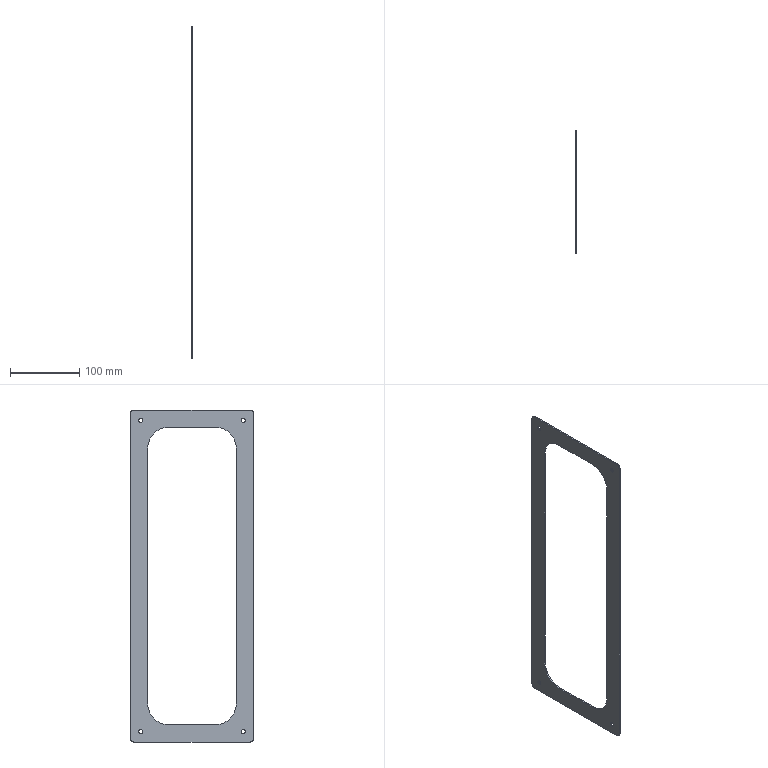Part | SolidWorks | features Fillet 2, ICE 2, Extrusion 1 | 1 solid | 26 faces | box 2 x 178 x 480 mm | volume 62076 mm3 | cylinder 16 | plane 10 | commonest cylinder face diameters 6 x8 10 x4 60 x4
STEP:
#1=CARTESIAN_POINT('',(0.,-74.,-222.));
#2=VERTEX_POINT('',#1);
#3=CARTESIAN_POINT('',(0.,-74.,-228.));
#4=VERTEX_POINT('',#3);
#5=CARTESIAN_POINT('',(0.,-74.,-225.));
#6=DIRECTION('',(1.,0.,0.));
#7=DIRECTION('',(0.,0.,-1.));
#8=AXIS2_PLACEMENT_3D('',#5,#6,#7);
#9=CIRCLE('',#8,3.);
#10=EDGE_CURVE('',#2,#4,#9,.T.);
#11=ORIENTED_EDGE('',*,*,#10,.F.);
#12=CARTESIAN_POINT('',(2.,-74.,-222.));
#13=VERTEX_POINT('',#12);
#14=CARTESIAN_POINT('',(0.,-74.,-222.));
#15=DIRECTION('',(1.,0.,0.));
#16=VECTOR('',#15,1000.);
#17=LINE('',#14,#16);
#18=EDGE_CURVE('',#2,#13,#17,.T.);
#19=ORIENTED_EDGE('',*,*,#18,.T.);
#20=CARTESIAN_POINT('',(2.,-74.,-228.));
#21=VERTEX_POINT('',#20);
#22=CARTESIAN_POINT('',(2.,-74.,-225.));
#23=DIRECTION('',(1.,0.,0.));
#24=DIRECTION('',(0.,0.,-1.));
#25=AXIS2_PLACEMENT_3D('',#22,#23,#24);
#26=CIRCLE('',#25,3.);
#27=EDGE_CURVE('',#13,#21,#26,.T.);
#28=ORIENTED_EDGE('',*,*,#27,.T.);
#29=CARTESIAN_POINT('',(0.,-74.,-228.));
#30=DIRECTION('',(1.,0.,0.));
#31=VECTOR('',#30,1000.);
#32=LINE('',#29,#31);
#33=EDGE_CURVE('',#4,#21,#32,.T.);
#34=ORIENTED_EDGE('',*,*,#33,.F.);
#35=EDGE_LOOP('',(#11,#19,#28,#34));
#36=FACE_OUTER_BOUND('',#35,.T.);
#37=CARTESIAN_POINT('',(0.,-74.,-225.));
#38=DIRECTION('',(1.,0.,0.));
#39=DIRECTION('',(0.,0.,-1.));
#40=AXIS2_PLACEMENT_3D('',#37,#38,#39);
#41=CYLINDRICAL_SURFACE('',#40,3.);
#42=ADVANCED_FACE('',(#36),#41,.F.);
#43=CARTESIAN_POINT('',(0.,-74.,228.));
#44=VERTEX_POINT('',#43);
#45=CARTESIAN_POINT('',(0.,-74.,222.));
#46=VERTEX_POINT('',#45);
#47=CARTESIAN_POINT('',(0.,-74.,225.));
#48=DIRECTION('',(1.,0.,0.));
#49=DIRECTION('',(0.,0.,-1.));
#50=AXIS2_PLACEMENT_3D('',#47,#48,#49);
#51=CIRCLE('',#50,3.);
#52=EDGE_CURVE('',#44,#46,#51,.T.);
#53=ORIENTED_EDGE('',*,*,#52,.F.);
#54=CARTESIAN_POINT('',(2.,-74.,228.));
#55=VERTEX_POINT('',#54);
#56=CARTESIAN_POINT('',(0.,-74.,228.));
#57=DIRECTION('',(1.,0.,0.));
#58=VECTOR('',#57,1000.);
#59=LINE('',#56,#58);
#60=EDGE_CURVE('',#44,#55,#59,.T.);
#61=ORIENTED_EDGE('',*,*,#60,.T.);
#62=CARTESIAN_POINT('',(2.,-74.,222.));
#63=VERTEX_POINT('',#62);
#64=CARTESIAN_POINT('',(2.,-74.,225.));
#65=DIRECTION('',(1.,0.,0.));
#66=DIRECTION('',(0.,0.,-1.));
#67=AXIS2_PLACEMENT_3D('',#64,#65,#66);
#68=CIRCLE('',#67,3.);
#69=EDGE_CURVE('',#55,#63,#68,.T.);
#70=ORIENTED_EDGE('',*,*,#69,.T.);
#71=CARTESIAN_POINT('',(0.,-74.,222.));
#72=DIRECTION('',(1.,0.,0.));
#73=VECTOR('',#72,1000.);
#74=LINE('',#71,#73);
#75=EDGE_CURVE('',#46,#63,#74,.T.);
#76=ORIENTED_EDGE('',*,*,#75,.F.);
#77=EDGE_LOOP('',(#53,#61,#70,#76));
#78=FACE_OUTER_BOUND('',#77,.T.);
#79=CARTESIAN_POINT('',(0.,-74.,225.));
#80=DIRECTION('',(1.,0.,0.));
#81=DIRECTION('',(0.,0.,-1.));
#82=AXIS2_PLACEMENT_3D('',#79,#80,#81);
#83=CYLINDRICAL_SURFACE('',#82,3.);
#84=ADVANCED_FACE('',(#78),#83,.F.);
#85=CARTESIAN_POINT('',(0.,74.,-222.));
#86=VERTEX_POINT('',#85);
#87=CARTESIAN_POINT('',(0.,74.,-228.));
#88=VERTEX_POINT('',#87);
#89=CARTESIAN_POINT('',(0.,74.,-225.));
#90=DIRECTION('',(1.,0.,0.));
#91=DIRECTION('',(0.,0.,-1.));
#92=AXIS2_PLACEMENT_3D('',#89,#90,#91);
#93=CIRCLE('',#92,3.);
#94=EDGE_CURVE('',#86,#88,#93,.T.);
#95=ORIENTED_EDGE('',*,*,#94,.F.);
#96=CARTESIAN_POINT('',(2.,74.,-222.));
#97=VERTEX_POINT('',#96);
#98=CARTESIAN_POINT('',(0.,74.,-222.));
#99=DIRECTION('',(1.,0.,0.));
#100=VECTOR('',#99,1000.);
#101=LINE('',#98,#100);
#102=EDGE_CURVE('',#86,#97,#101,.T.);
#103=ORIENTED_EDGE('',*,*,#102,.T.);
#104=CARTESIAN_POINT('',(2.,74.,-228.));
#105=VERTEX_POINT('',#104);
#106=CARTESIAN_POINT('',(2.,74.,-225.));
#107=DIRECTION('',(1.,0.,0.));
#108=DIRECTION('',(0.,0.,-1.));
#109=AXIS2_PLACEMENT_3D('',#106,#107,#108);
#110=CIRCLE('',#109,3.);
#111=EDGE_CURVE('',#97,#105,#110,.T.);
#112=ORIENTED_EDGE('',*,*,#111,.T.);
#113=CARTESIAN_POINT('',(0.,74.,-228.));
#114=DIRECTION('',(1.,0.,0.));
#115=VECTOR('',#114,1000.);
#116=LINE('',#113,#115);
#117=EDGE_CURVE('',#88,#105,#116,.T.);
#118=ORIENTED_EDGE('',*,*,#117,.F.);
#119=EDGE_LOOP('',(#95,#103,#112,#118));
#120=FACE_OUTER_BOUND('',#119,.T.);
#121=CARTESIAN_POINT('',(0.,74.,-225.));
#122=DIRECTION('',(1.,0.,0.));
#123=DIRECTION('',(0.,0.,-1.));
#124=AXIS2_PLACEMENT_3D('',#121,#122,#123);
#125=CYLINDRICAL_SURFACE('',#124,3.);
#126=ADVANCED_FACE('',(#120),#125,.F.);
#127=CARTESIAN_POINT('',(0.,74.,228.));
#128=VERTEX_POINT('',#127);
#129=CARTESIAN_POINT('',(0.,74.,222.));
#130=VERTEX_POINT('',#129);
#131=CARTESIAN_POINT('',(0.,74.,225.));
#132=DIRECTION('',(1.,0.,0.));
#133=DIRECTION('',(0.,0.,-1.));
#134=AXIS2_PLACEMENT_3D('',#131,#132,#133);
#135=CIRCLE('',#134,3.);
#136=EDGE_CURVE('',#128,#130,#135,.T.);
#137=ORIENTED_EDGE('',*,*,#136,.F.);
#138=CARTESIAN_POINT('',(2.,74.,228.));
#139=VERTEX_POINT('',#138);
#140=CARTESIAN_POINT('',(0.,74.,228.));
#141=DIRECTION('',(1.,0.,0.));
#142=VECTOR('',#141,1000.);
#143=LINE('',#140,#142);
#144=EDGE_CURVE('',#128,#139,#143,.T.);
#145=ORIENTED_EDGE('',*,*,#144,.T.);
#146=CARTESIAN_POINT('',(2.,74.,222.));
#147=VERTEX_POINT('',#146);
#148=CARTESIAN_POINT('',(2.,74.,225.));
#149=DIRECTION('',(1.,0.,0.));
#150=DIRECTION('',(0.,0.,-1.));
#151=AXIS2_PLACEMENT_3D('',#148,#149,#150);
#152=CIRCLE('',#151,3.);
#153=EDGE_CURVE('',#139,#147,#152,.T.);
#154=ORIENTED_EDGE('',*,*,#153,.T.);
#155=CARTESIAN_POINT('',(0.,74.,222.));
#156=DIRECTION('',(1.,0.,0.));
#157=VECTOR('',#156,1000.);
#158=LINE('',#155,#157);
#159=EDGE_CURVE('',#130,#147,#158,.T.);
#160=ORIENTED_EDGE('',*,*,#159,.F.);
#161=EDGE_LOOP('',(#137,#145,#154,#160));
#162=FACE_OUTER_BOUND('',#161,.T.);
#163=CARTESIAN_POINT('',(0.,74.,225.));
#164=DIRECTION('',(1.,0.,0.));
#165=DIRECTION('',(0.,0.,-1.));
#166=AXIS2_PLACEMENT_3D('',#163,#164,#165);
#167=CYLINDRICAL_SURFACE('',#166,3.);
#168=ADVANCED_FACE('',(#162),#167,.F.);
#169=CARTESIAN_POINT('',(0.,84.,240.));
#170=VERTEX_POINT('',#169);
#171=CARTESIAN_POINT('',(0.,-84.,240.));
#172=VERTEX_POINT('',#171);
#173=CARTESIAN_POINT('',(0.,89.,240.));
#174=DIRECTION('',(0.,-1.,0.));
#175=VECTOR('',#174,1000.);
#176=LINE('',#173,#175);
#177=EDGE_CURVE('',#170,#172,#176,.T.);
#178=ORIENTED_EDGE('',*,*,#177,.T.);
#179=CARTESIAN_POINT('',(2.,-84.,240.));
#180=VERTEX_POINT('',#179);
#181=CARTESIAN_POINT('',(2.,-84.,240.));
#182=DIRECTION('',(1.,0.,0.));
#183=VECTOR('',#182,1000.);
#184=LINE('',#181,#183);
#185=EDGE_CURVE('',#172,#180,#184,.T.);
#186=ORIENTED_EDGE('',*,*,#185,.T.);
#187=CARTESIAN_POINT('',(2.,84.,240.));
#188=VERTEX_POINT('',#187);
#189=CARTESIAN_POINT('',(2.,89.,240.));
#190=DIRECTION('',(0.,-1.,0.));
#191=VECTOR('',#190,1000.);
#192=LINE('',#189,#191);
#193=EDGE_CURVE('',#188,#180,#192,.T.);
#194=ORIENTED_EDGE('',*,*,#193,.F.);
#195=CARTESIAN_POINT('',(2.,84.,240.));
#196=DIRECTION('',(-1.,0.,0.));
#197=VECTOR('',#196,1000.);
#198=LINE('',#195,#197);
#199=EDGE_CURVE('',#188,#170,#198,.T.);
#200=ORIENTED_EDGE('',*,*,#199,.T.);
#201=EDGE_LOOP('',(#178,#186,#194,#200));
#202=FACE_OUTER_BOUND('',#201,.T.);
#203=CARTESIAN_POINT('',(2.,89.,240.));
#204=DIRECTION('',(0.,0.,-1.));
#205=DIRECTION('',(-1.,0.,0.));
#206=AXIS2_PLACEMENT_3D('',#203,#204,#205);
#207=PLANE('',#206);
#208=ADVANCED_FACE('',(#202),#207,.F.);
#209=CARTESIAN_POINT('',(2.,-89.,235.));
#210=VERTEX_POINT('',#209);
#211=CARTESIAN_POINT('',(2.,-89.,-235.));
#212=VERTEX_POINT('',#211);
#213=CARTESIAN_POINT('',(2.,-89.,240.));
#214=DIRECTION('',(0.,0.,-1.));
#215=VECTOR('',#214,1000.);
#216=LINE('',#213,#215);
#217=EDGE_CURVE('',#210,#212,#216,.T.);
#218=ORIENTED_EDGE('',*,*,#217,.F.);
#219=CARTESIAN_POINT('',(0.,-89.,235.));
#220=VERTEX_POINT('',#219);
#221=CARTESIAN_POINT('',(2.,-89.,235.));
#222=DIRECTION('',(-1.,0.,0.));
#223=VECTOR('',#222,1000.);
#224=LINE('',#221,#223);
#225=EDGE_CURVE('',#210,#220,#224,.T.);
#226=ORIENTED_EDGE('',*,*,#225,.T.);
#227=CARTESIAN_POINT('',(0.,-89.,-235.));
#228=VERTEX_POINT('',#227);
#229=CARTESIAN_POINT('',(0.,-89.,240.));
#230=DIRECTION('',(0.,0.,-1.));
#231=VECTOR('',#230,1000.);
#232=LINE('',#229,#231);
#233=EDGE_CURVE('',#220,#228,#232,.T.);
#234=ORIENTED_EDGE('',*,*,#233,.T.);
#235=CARTESIAN_POINT('',(2.,-89.,-235.));
#236=DIRECTION('',(1.,0.,0.));
#237=VECTOR('',#236,1000.);
#238=LINE('',#235,#237);
#239=EDGE_CURVE('',#228,#212,#238,.T.);
#240=ORIENTED_EDGE('',*,*,#239,.T.);
#241=EDGE_LOOP('',(#218,#226,#234,#240));
#242=FACE_OUTER_BOUND('',#241,.T.);
#243=CARTESIAN_POINT('',(2.,-89.,240.));
#244=DIRECTION('',(0.,1.,0.));
#245=DIRECTION('',(0.,0.,1.));
#246=AXIS2_PLACEMENT_3D('',#243,#244,#245);
#247=PLANE('',#246);
#248=ADVANCED_FACE('',(#242),#247,.F.);
#249=CARTESIAN_POINT('',(2.,-84.,-240.));
#250=VERTEX_POINT('',#249);
#251=CARTESIAN_POINT('',(2.,84.,-240.));
#252=VERTEX_POINT('',#251);
#253=CARTESIAN_POINT('',(2.,89.,-240.));
#254=DIRECTION('',(0.,1.,0.));
#255=VECTOR('',#254,1000.);
#256=LINE('',#253,#255);
#257=EDGE_CURVE('',#250,#252,#256,.T.);
#258=ORIENTED_EDGE('',*,*,#257,.F.);
#259=CARTESIAN_POINT('',(0.,-84.,-240.));
#260=VERTEX_POINT('',#259);
#261=CARTESIAN_POINT('',(2.,-84.,-240.));
#262=DIRECTION('',(-1.,0.,0.));
#263=VECTOR('',#262,1000.);
#264=LINE('',#261,#263);
#265=EDGE_CURVE('',#250,#260,#264,.T.);
#266=ORIENTED_EDGE('',*,*,#265,.T.);
#267=CARTESIAN_POINT('',(0.,84.,-240.));
#268=VERTEX_POINT('',#267);
#269=CARTESIAN_POINT('',(0.,89.,-240.));
#270=DIRECTION('',(0.,1.,0.));
#271=VECTOR('',#270,1000.);
#272=LINE('',#269,#271);
#273=EDGE_CURVE('',#260,#268,#272,.T.);
#274=ORIENTED_EDGE('',*,*,#273,.T.);
#275=CARTESIAN_POINT('',(2.,84.,-240.));
#276=DIRECTION('',(1.,0.,0.));
#277=VECTOR('',#276,1000.);
#278=LINE('',#275,#277);
#279=EDGE_CURVE('',#268,#252,#278,.T.);
#280=ORIENTED_EDGE('',*,*,#279,.T.);
#281=EDGE_LOOP('',(#258,#266,#274,#280));
#282=FACE_OUTER_BOUND('',#281,.T.);
#283=CARTESIAN_POINT('',(2.,89.,-240.));
#284=DIRECTION('',(0.,0.,1.));
#285=DIRECTION('',(1.,0.,0.));
#286=AXIS2_PLACEMENT_3D('',#283,#284,#285);
#287=PLANE('',#286);
#288=ADVANCED_FACE('',(#282),#287,.F.);
#289=CARTESIAN_POINT('',(2.,89.,-235.));
#290=VERTEX_POINT('',#289);
#291=CARTESIAN_POINT('',(2.,89.,235.));
#292=VERTEX_POINT('',#291);
#293=CARTESIAN_POINT('',(2.,89.,240.));
#294=DIRECTION('',(0.,0.,1.));
#295=VECTOR('',#294,1000.);
#296=LINE('',#293,#295);
#297=EDGE_CURVE('',#290,#292,#296,.T.);
#298=ORIENTED_EDGE('',*,*,#297,.F.);
#299=CARTESIAN_POINT('',(0.,89.,-235.));
#300=VERTEX_POINT('',#299);
#301=CARTESIAN_POINT('',(2.,89.,-235.));
#302=DIRECTION('',(-1.,0.,0.));
#303=VECTOR('',#302,1000.);
#304=LINE('',#301,#303);
#305=EDGE_CURVE('',#290,#300,#304,.T.);
#306=ORIENTED_EDGE('',*,*,#305,.T.);
#307=CARTESIAN_POINT('',(0.,89.,235.));
#308=VERTEX_POINT('',#307);
#309=CARTESIAN_POINT('',(0.,89.,240.));
#310=DIRECTION('',(0.,0.,1.));
#311=VECTOR('',#310,1000.);
#312=LINE('',#309,#311);
#313=EDGE_CURVE('',#300,#308,#312,.T.);
#314=ORIENTED_EDGE('',*,*,#313,.T.);
#315=CARTESIAN_POINT('',(2.,89.,235.));
#316=DIRECTION('',(1.,0.,0.));
#317=VECTOR('',#316,1000.);
#318=LINE('',#315,#317);
#319=EDGE_CURVE('',#308,#292,#318,.T.);
#320=ORIENTED_EDGE('',*,*,#319,.T.);
#321=EDGE_LOOP('',(#298,#306,#314,#320));
#322=FACE_OUTER_BOUND('',#321,.T.);
#323=CARTESIAN_POINT('',(2.,89.,240.));
#324=DIRECTION('',(0.,-1.,0.));
#325=DIRECTION('',(0.,0.,-1.));
#326=AXIS2_PLACEMENT_3D('',#323,#324,#325);
#327=PLANE('',#326);
#328=ADVANCED_FACE('',(#322),#327,.F.);
#329=CARTESIAN_POINT('',(2.,34.,215.));
#330=VERTEX_POINT('',#329);
#331=CARTESIAN_POINT('',(2.,-34.,215.));
#332=VERTEX_POINT('',#331);
#333=CARTESIAN_POINT('',(2.,64.,215.));
#334=DIRECTION('',(0.,-1.,0.));
#335=VECTOR('',#334,1000.);
#336=LINE('',#333,#335);
#337=EDGE_CURVE('',#330,#332,#336,.T.);
#338=ORIENTED_EDGE('',*,*,#337,.F.);
#339=CARTESIAN_POINT('',(2.,64.,185.));
#340=VERTEX_POINT('',#339);
#341=CARTESIAN_POINT('',(2.,34.,185.));
#342=DIRECTION('',(-1.,0.,0.));
#343=DIRECTION('',(0.,0.,-1.));
#344=AXIS2_PLACEMENT_3D('',#341,#342,#343);
#345=CIRCLE('',#344,30.);
#346=EDGE_CURVE('',#330,#340,#345,.T.);
#347=ORIENTED_EDGE('',*,*,#346,.T.);
#348=CARTESIAN_POINT('',(2.,64.,-185.));
#349=VERTEX_POINT('',#348);
#350=CARTESIAN_POINT('',(2.,64.,215.));
#351=DIRECTION('',(0.,0.,1.));
#352=VECTOR('',#351,1000.);
#353=LINE('',#350,#352);
#354=EDGE_CURVE('',#349,#340,#353,.T.);
#355=ORIENTED_EDGE('',*,*,#354,.F.);
#356=CARTESIAN_POINT('',(2.,34.,-215.));
#357=VERTEX_POINT('',#356);
#358=CARTESIAN_POINT('',(2.,34.,-185.));
#359=DIRECTION('',(-1.,0.,0.));
#360=DIRECTION('',(0.,0.,-1.));
#361=AXIS2_PLACEMENT_3D('',#358,#359,#360);
#362=CIRCLE('',#361,30.);
#363=EDGE_CURVE('',#349,#357,#362,.T.);
#364=ORIENTED_EDGE('',*,*,#363,.T.);
#365=CARTESIAN_POINT('',(2.,-34.,-215.));
#366=VERTEX_POINT('',#365);
#367=CARTESIAN_POINT('',(2.,64.,-215.));
#368=DIRECTION('',(0.,1.,0.));
#369=VECTOR('',#368,1000.);
#370=LINE('',#367,#369);
#371=EDGE_CURVE('',#366,#357,#370,.T.);
#372=ORIENTED_EDGE('',*,*,#371,.F.);
#373=CARTESIAN_POINT('',(2.,-64.,-185.));
#374=VERTEX_POINT('',#373);
#375=CARTESIAN_POINT('',(2.,-34.,-185.));
#376=DIRECTION('',(-1.,0.,0.));
#377=DIRECTION('',(0.,0.,-1.));
#378=AXIS2_PLACEMENT_3D('',#375,#376,#377);
#379=CIRCLE('',#378,30.);
#380=EDGE_CURVE('',#366,#374,#379,.T.);
#381=ORIENTED_EDGE('',*,*,#380,.T.);
#382=CARTESIAN_POINT('',(2.,-64.,185.));
#383=VERTEX_POINT('',#382);
#384=CARTESIAN_POINT('',(2.,-64.,215.));
#385=DIRECTION('',(0.,0.,-1.));
#386=VECTOR('',#385,1000.);
#387=LINE('',#384,#386);
#388=EDGE_CURVE('',#383,#374,#387,.T.);
#389=ORIENTED_EDGE('',*,*,#388,.F.);
#390=CARTESIAN_POINT('',(2.,-34.,185.));
#391=DIRECTION('',(-1.,0.,0.));
#392=DIRECTION('',(0.,0.,-1.));
#393=AXIS2_PLACEMENT_3D('',#390,#391,#392);
#394=CIRCLE('',#393,30.);
#395=EDGE_CURVE('',#383,#332,#394,.T.);
#396=ORIENTED_EDGE('',*,*,#395,.T.);
#397=EDGE_LOOP('',(#338,#347,#355,#364,#372,#381,#389,#396));
#398=FACE_BOUND('',#397,.T.);
#399=CARTESIAN_POINT('',(2.,-74.,-225.));
#400=DIRECTION('',(1.,0.,0.));
#401=DIRECTION('',(0.,0.,-1.));
#402=AXIS2_PLACEMENT_3D('',#399,#400,#401);
#403=CIRCLE('',#402,3.);
#404=EDGE_CURVE('',#21,#13,#403,.T.);
#405=ORIENTED_EDGE('',*,*,#404,.F.);
#406=ORIENTED_EDGE('',*,*,#27,.F.);
#407=EDGE_LOOP('',(#405,#406));
#408=FACE_BOUND('',#407,.T.);
#409=CARTESIAN_POINT('',(2.,-74.,225.));
#410=DIRECTION('',(1.,0.,0.));
#411=DIRECTION('',(0.,0.,-1.));
#412=AXIS2_PLACEMENT_3D('',#409,#410,#411);
#413=CIRCLE('',#412,3.);
#414=EDGE_CURVE('',#63,#55,#413,.T.);
#415=ORIENTED_EDGE('',*,*,#414,.F.);
#416=ORIENTED_EDGE('',*,*,#69,.F.);
#417=EDGE_LOOP('',(#415,#416));
#418=FACE_BOUND('',#417,.T.);
#419=CARTESIAN_POINT('',(2.,74.,-225.));
#420=DIRECTION('',(1.,0.,0.));
#421=DIRECTION('',(0.,0.,-1.));
#422=AXIS2_PLACEMENT_3D('',#419,#420,#421);
#423=CIRCLE('',#422,3.);
#424=EDGE_CURVE('',#105,#97,#423,.T.);
#425=ORIENTED_EDGE('',*,*,#424,.F.);
#426=ORIENTED_EDGE('',*,*,#111,.F.);
#427=EDGE_LOOP('',(#425,#426));
#428=FACE_BOUND('',#427,.T.);
#429=CARTESIAN_POINT('',(2.,74.,225.));
#430=DIRECTION('',(1.,0.,0.));
#431=DIRECTION('',(0.,0.,-1.));
#432=AXIS2_PLACEMENT_3D('',#429,#430,#431);
#433=CIRCLE('',#432,3.);
#434=EDGE_CURVE('',#147,#139,#433,.T.);
#435=ORIENTED_EDGE('',*,*,#434,.F.);
#436=ORIENTED_EDGE('',*,*,#153,.F.);
#437=EDGE_LOOP('',(#435,#436));
#438=FACE_BOUND('',#437,.T.);
#439=ORIENTED_EDGE('',*,*,#193,.T.);
#440=CARTESIAN_POINT('',(2.,-84.,235.));
#441=DIRECTION('',(1.,0.,0.));
#442=DIRECTION('',(0.,0.,-1.));
#443=AXIS2_PLACEMENT_3D('',#440,#441,#442);
#444=CIRCLE('',#443,5.);
#445=EDGE_CURVE('',#180,#210,#444,.T.);
#446=ORIENTED_EDGE('',*,*,#445,.T.);
#447=ORIENTED_EDGE('',*,*,#217,.T.);
#448=CARTESIAN_POINT('',(2.,-84.,-235.));
#449=DIRECTION('',(1.,0.,0.));
#450=DIRECTION('',(0.,0.,-1.));
#451=AXIS2_PLACEMENT_3D('',#448,#449,#450);
#452=CIRCLE('',#451,5.);
#453=EDGE_CURVE('',#212,#250,#452,.T.);
#454=ORIENTED_EDGE('',*,*,#453,.T.);
#455=ORIENTED_EDGE('',*,*,#257,.T.);
#456=CARTESIAN_POINT('',(2.,84.,-235.));
#457=DIRECTION('',(1.,0.,0.));
#458=DIRECTION('',(0.,0.,-1.));
#459=AXIS2_PLACEMENT_3D('',#456,#457,#458);
#460=CIRCLE('',#459,5.);
#461=EDGE_CURVE('',#252,#290,#460,.T.);
#462=ORIENTED_EDGE('',*,*,#461,.T.);
#463=ORIENTED_EDGE('',*,*,#297,.T.);
#464=CARTESIAN_POINT('',(2.,84.,235.));
#465=DIRECTION('',(1.,0.,0.));
#466=DIRECTION('',(0.,0.,-1.));
#467=AXIS2_PLACEMENT_3D('',#464,#465,#466);
#468=CIRCLE('',#467,5.);
#469=EDGE_CURVE('',#292,#188,#468,.T.);
#470=ORIENTED_EDGE('',*,*,#469,.T.);
#471=EDGE_LOOP('',(#439,#446,#447,#454,#455,#462,#463,#470));
#472=FACE_OUTER_BOUND('',#471,.T.);
#473=CARTESIAN_POINT('',(2.,0.,0.));
#474=DIRECTION('',(1.,0.,0.));
#475=DIRECTION('',(0.,0.,-1.));
#476=AXIS2_PLACEMENT_3D('',#473,#474,#475);
#477=PLANE('',#476);
#478=ADVANCED_FACE('',(#398,#408,#418,#428,#438,#472),#477,.T.);
#479=CARTESIAN_POINT('',(0.,-34.,-215.));
#480=VERTEX_POINT('',#479);
#481=CARTESIAN_POINT('',(0.,34.,-215.));
#482=VERTEX_POINT('',#481);
#483=CARTESIAN_POINT('',(0.,64.,-215.));
#484=DIRECTION('',(0.,1.,0.));
#485=VECTOR('',#484,1000.);
#486=LINE('',#483,#485);
#487=EDGE_CURVE('',#480,#482,#486,.T.);
#488=ORIENTED_EDGE('',*,*,#487,.T.);
#489=CARTESIAN_POINT('',(0.,64.,-185.));
#490=VERTEX_POINT('',#489);
#491=CARTESIAN_POINT('',(0.,34.,-185.));
#492=DIRECTION('',(1.,0.,0.));
#493=DIRECTION('',(0.,0.,-1.));
#494=AXIS2_PLACEMENT_3D('',#491,#492,#493);
#495=CIRCLE('',#494,30.);
#496=EDGE_CURVE('',#482,#490,#495,.T.);
#497=ORIENTED_EDGE('',*,*,#496,.T.);
#498=CARTESIAN_POINT('',(0.,64.,185.));
#499=VERTEX_POINT('',#498);
#500=CARTESIAN_POINT('',(0.,64.,215.));
#501=DIRECTION('',(0.,0.,1.));
#502=VECTOR('',#501,1000.);
#503=LINE('',#500,#502);
#504=EDGE_CURVE('',#490,#499,#503,.T.);
#505=ORIENTED_EDGE('',*,*,#504,.T.);
#506=CARTESIAN_POINT('',(0.,34.,215.));
#507=VERTEX_POINT('',#506);
#508=CARTESIAN_POINT('',(0.,34.,185.));
#509=DIRECTION('',(1.,0.,0.));
#510=DIRECTION('',(0.,0.,-1.));
#511=AXIS2_PLACEMENT_3D('',#508,#509,#510);
#512=CIRCLE('',#511,30.);
#513=EDGE_CURVE('',#499,#507,#512,.T.);
#514=ORIENTED_EDGE('',*,*,#513,.T.);
#515=CARTESIAN_POINT('',(0.,-34.,215.));
#516=VERTEX_POINT('',#515);
#517=CARTESIAN_POINT('',(0.,64.,215.));
#518=DIRECTION('',(0.,-1.,0.));
#519=VECTOR('',#518,1000.);
#520=LINE('',#517,#519);
#521=EDGE_CURVE('',#507,#516,#520,.T.);
#522=ORIENTED_EDGE('',*,*,#521,.T.);
#523=CARTESIAN_POINT('',(0.,-64.,185.));
#524=VERTEX_POINT('',#523);
#525=CARTESIAN_POINT('',(0.,-34.,185.));
#526=DIRECTION('',(1.,0.,0.));
#527=DIRECTION('',(0.,0.,-1.));
#528=AXIS2_PLACEMENT_3D('',#525,#526,#527);
#529=CIRCLE('',#528,30.);
#530=EDGE_CURVE('',#516,#524,#529,.T.);
#531=ORIENTED_EDGE('',*,*,#530,.T.);
#532=CARTESIAN_POINT('',(0.,-64.,-185.));
#533=VERTEX_POINT('',#532);
#534=CARTESIAN_POINT('',(0.,-64.,215.));
#535=DIRECTION('',(0.,0.,-1.));
#536=VECTOR('',#535,1000.);
#537=LINE('',#534,#536);
#538=EDGE_CURVE('',#524,#533,#537,.T.);
#539=ORIENTED_EDGE('',*,*,#538,.T.);
#540=CARTESIAN_POINT('',(0.,-34.,-185.));
#541=DIRECTION('',(1.,0.,0.));
#542=DIRECTION('',(0.,0.,-1.));
#543=AXIS2_PLACEMENT_3D('',#540,#541,#542);
#544=CIRCLE('',#543,30.);
#545=EDGE_CURVE('',#533,#480,#544,.T.);
#546=ORIENTED_EDGE('',*,*,#545,.T.);
#547=EDGE_LOOP('',(#488,#497,#505,#514,#522,#531,#539,#546));
#548=FACE_BOUND('',#547,.T.);
#549=CARTESIAN_POINT('',(0.,-74.,-225.));
#550=DIRECTION('',(1.,0.,0.));
#551=DIRECTION('',(0.,0.,-1.));
#552=AXIS2_PLACEMENT_3D('',#549,#550,#551);
#553=CIRCLE('',#552,3.);
#554=EDGE_CURVE('',#4,#2,#553,.T.);
#555=ORIENTED_EDGE('',*,*,#554,.T.);
#556=ORIENTED_EDGE('',*,*,#10,.T.);
#557=EDGE_LOOP('',(#555,#556));
#558=FACE_BOUND('',#557,.T.);
#559=CARTESIAN_POINT('',(0.,-74.,225.));
#560=DIRECTION('',(1.,0.,0.));
#561=DIRECTION('',(0.,0.,-1.));
#562=AXIS2_PLACEMENT_3D('',#559,#560,#561);
#563=CIRCLE('',#562,3.);
#564=EDGE_CURVE('',#46,#44,#563,.T.);
#565=ORIENTED_EDGE('',*,*,#564,.T.);
#566=ORIENTED_EDGE('',*,*,#52,.T.);
#567=EDGE_LOOP('',(#565,#566));
#568=FACE_BOUND('',#567,.T.);
#569=CARTESIAN_POINT('',(0.,74.,-225.));
#570=DIRECTION('',(1.,0.,0.));
#571=DIRECTION('',(0.,0.,-1.));
#572=AXIS2_PLACEMENT_3D('',#569,#570,#571);
#573=CIRCLE('',#572,3.);
#574=EDGE_CURVE('',#88,#86,#573,.T.);
#575=ORIENTED_EDGE('',*,*,#574,.T.);
#576=ORIENTED_EDGE('',*,*,#94,.T.);
#577=EDGE_LOOP('',(#575,#576));
#578=FACE_BOUND('',#577,.T.);
#579=CARTESIAN_POINT('',(0.,74.,225.));
#580=DIRECTION('',(1.,0.,0.));
#581=DIRECTION('',(0.,0.,-1.));
#582=AXIS2_PLACEMENT_3D('',#579,#580,#581);
#583=CIRCLE('',#582,3.);
#584=EDGE_CURVE('',#130,#128,#583,.T.);
#585=ORIENTED_EDGE('',*,*,#584,.T.);
#586=ORIENTED_EDGE('',*,*,#136,.T.);
#587=EDGE_LOOP('',(#585,#586));
#588=FACE_BOUND('',#587,.T.);
#589=ORIENTED_EDGE('',*,*,#233,.F.);
#590=CARTESIAN_POINT('',(0.,-84.,235.));
#591=DIRECTION('',(-1.,0.,0.));
#592=DIRECTION('',(0.,0.,-1.));
#593=AXIS2_PLACEMENT_3D('',#590,#591,#592);
#594=CIRCLE('',#593,5.);
#595=EDGE_CURVE('',#220,#172,#594,.T.);
#596=ORIENTED_EDGE('',*,*,#595,.T.);
#597=ORIENTED_EDGE('',*,*,#177,.F.);
#598=CARTESIAN_POINT('',(0.,84.,235.));
#599=DIRECTION('',(-1.,0.,0.));
#600=DIRECTION('',(0.,0.,-1.));
#601=AXIS2_PLACEMENT_3D('',#598,#599,#600);
#602=CIRCLE('',#601,5.);
#603=EDGE_CURVE('',#170,#308,#602,.T.);
#604=ORIENTED_EDGE('',*,*,#603,.T.);
#605=ORIENTED_EDGE('',*,*,#313,.F.);
#606=CARTESIAN_POINT('',(0.,84.,-235.));
#607=DIRECTION('',(-1.,0.,0.));
#608=DIRECTION('',(0.,0.,-1.));
#609=AXIS2_PLACEMENT_3D('',#606,#607,#608);
#610=CIRCLE('',#609,5.);
#611=EDGE_CURVE('',#300,#268,#610,.T.);
#612=ORIENTED_EDGE('',*,*,#611,.T.);
#613=ORIENTED_EDGE('',*,*,#273,.F.);
#614=CARTESIAN_POINT('',(0.,-84.,-235.));
#615=DIRECTION('',(-1.,0.,0.));
#616=DIRECTION('',(0.,0.,-1.));
#617=AXIS2_PLACEMENT_3D('',#614,#615,#616);
#618=CIRCLE('',#617,5.);
#619=EDGE_CURVE('',#260,#228,#618,.T.);
#620=ORIENTED_EDGE('',*,*,#619,.T.);
#621=EDGE_LOOP('',(#589,#596,#597,#604,#605,#612,#613,#620));
#622=FACE_OUTER_BOUND('',#621,.T.);
#623=CARTESIAN_POINT('',(0.,0.,0.));
#624=DIRECTION('',(1.,0.,0.));
#625=DIRECTION('',(0.,0.,-1.));
#626=AXIS2_PLACEMENT_3D('',#623,#624,#625);
#627=PLANE('',#626);
#628=ADVANCED_FACE('',(#548,#558,#568,#578,#588,#622),#627,.F.);
#629=ORIENTED_EDGE('',*,*,#144,.F.);
#630=ORIENTED_EDGE('',*,*,#584,.F.);
#631=ORIENTED_EDGE('',*,*,#159,.T.);
#632=ORIENTED_EDGE('',*,*,#434,.T.);
#633=EDGE_LOOP('',(#629,#630,#631,#632));
#634=FACE_OUTER_BOUND('',#633,.T.);
#635=CARTESIAN_POINT('',(0.,74.,225.));
#636=DIRECTION('',(1.,0.,0.));
#637=DIRECTION('',(0.,0.,-1.));
#638=AXIS2_PLACEMENT_3D('',#635,#636,#637);
#639=CYLINDRICAL_SURFACE('',#638,3.);
#640=ADVANCED_FACE('',(#634),#639,.F.);
#641=ORIENTED_EDGE('',*,*,#102,.F.);
#642=ORIENTED_EDGE('',*,*,#574,.F.);
#643=ORIENTED_EDGE('',*,*,#117,.T.);
#644=ORIENTED_EDGE('',*,*,#424,.T.);
#645=EDGE_LOOP('',(#641,#642,#643,#644));
#646=FACE_OUTER_BOUND('',#645,.T.);
#647=CARTESIAN_POINT('',(0.,74.,-225.));
#648=DIRECTION('',(1.,0.,0.));
#649=DIRECTION('',(0.,0.,-1.));
#650=AXIS2_PLACEMENT_3D('',#647,#648,#649);
#651=CYLINDRICAL_SURFACE('',#650,3.);
#652=ADVANCED_FACE('',(#646),#651,.F.);
#653=ORIENTED_EDGE('',*,*,#60,.F.);
#654=ORIENTED_EDGE('',*,*,#564,.F.);
#655=ORIENTED_EDGE('',*,*,#75,.T.);
#656=ORIENTED_EDGE('',*,*,#414,.T.);
#657=EDGE_LOOP('',(#653,#654,#655,#656));
#658=FACE_OUTER_BOUND('',#657,.T.);
#659=CARTESIAN_POINT('',(0.,-74.,225.));
#660=DIRECTION('',(1.,0.,0.));
#661=DIRECTION('',(0.,0.,-1.));
#662=AXIS2_PLACEMENT_3D('',#659,#660,#661);
#663=CYLINDRICAL_SURFACE('',#662,3.);
#664=ADVANCED_FACE('',(#658),#663,.F.);
#665=ORIENTED_EDGE('',*,*,#18,.F.);
#666=ORIENTED_EDGE('',*,*,#554,.F.);
#667=ORIENTED_EDGE('',*,*,#33,.T.);
#668=ORIENTED_EDGE('',*,*,#404,.T.);
#669=EDGE_LOOP('',(#665,#666,#667,#668));
#670=FACE_OUTER_BOUND('',#669,.T.);
#671=CARTESIAN_POINT('',(0.,-74.,-225.));
#672=DIRECTION('',(1.,0.,0.));
#673=DIRECTION('',(0.,0.,-1.));
#674=AXIS2_PLACEMENT_3D('',#671,#672,#673);
#675=CYLINDRICAL_SURFACE('',#674,3.);
#676=ADVANCED_FACE('',(#670),#675,.F.);
#677=ORIENTED_EDGE('',*,*,#445,.F.);
#678=ORIENTED_EDGE('',*,*,#185,.F.);
#679=ORIENTED_EDGE('',*,*,#595,.F.);
#680=ORIENTED_EDGE('',*,*,#225,.F.);
#681=EDGE_LOOP('',(#677,#678,#679,#680));
#682=FACE_OUTER_BOUND('',#681,.T.);
#683=CARTESIAN_POINT('',(2.,-84.,235.));
#684=DIRECTION('',(-1.,0.,0.));
#685=DIRECTION('',(0.,0.,1.));
#686=AXIS2_PLACEMENT_3D('',#683,#684,#685);
#687=CYLINDRICAL_SURFACE('',#686,5.);
#688=ADVANCED_FACE('',(#682),#687,.T.);
#689=ORIENTED_EDGE('',*,*,#453,.F.);
#690=ORIENTED_EDGE('',*,*,#239,.F.);
#691=ORIENTED_EDGE('',*,*,#619,.F.);
#692=ORIENTED_EDGE('',*,*,#265,.F.);
#693=EDGE_LOOP('',(#689,#690,#691,#692));
#694=FACE_OUTER_BOUND('',#693,.T.);
#695=CARTESIAN_POINT('',(2.,-84.,-235.));
#696=DIRECTION('',(-1.,0.,0.));
#697=DIRECTION('',(0.,0.,1.));
#698=AXIS2_PLACEMENT_3D('',#695,#696,#697);
#699=CYLINDRICAL_SURFACE('',#698,5.);
#700=ADVANCED_FACE('',(#694),#699,.T.);
#701=ORIENTED_EDGE('',*,*,#461,.F.);
#702=ORIENTED_EDGE('',*,*,#279,.F.);
#703=ORIENTED_EDGE('',*,*,#611,.F.);
#704=ORIENTED_EDGE('',*,*,#305,.F.);
#705=EDGE_LOOP('',(#701,#702,#703,#704));
#706=FACE_OUTER_BOUND('',#705,.T.);
#707=CARTESIAN_POINT('',(2.,84.,-235.));
#708=DIRECTION('',(-1.,0.,0.));
#709=DIRECTION('',(0.,0.,1.));
#710=AXIS2_PLACEMENT_3D('',#707,#708,#709);
#711=CYLINDRICAL_SURFACE('',#710,5.);
#712=ADVANCED_FACE('',(#706),#711,.T.);
#713=ORIENTED_EDGE('',*,*,#469,.F.);
#714=ORIENTED_EDGE('',*,*,#319,.F.);
#715=ORIENTED_EDGE('',*,*,#603,.F.);
#716=ORIENTED_EDGE('',*,*,#199,.F.);
#717=EDGE_LOOP('',(#713,#714,#715,#716));
#718=FACE_OUTER_BOUND('',#717,.T.);
#719=CARTESIAN_POINT('',(2.,84.,235.));
#720=DIRECTION('',(-1.,0.,0.));
#721=DIRECTION('',(0.,0.,1.));
#722=AXIS2_PLACEMENT_3D('',#719,#720,#721);
#723=CYLINDRICAL_SURFACE('',#722,5.);
#724=ADVANCED_FACE('',(#718),#723,.T.);
#725=ORIENTED_EDGE('',*,*,#337,.T.);
#726=CARTESIAN_POINT('',(0.,-34.,215.));
#727=DIRECTION('',(-1.,0.,0.));
#728=VECTOR('',#727,1000.);
#729=LINE('',#726,#728);
#730=EDGE_CURVE('',#332,#516,#729,.T.);
#731=ORIENTED_EDGE('',*,*,#730,.T.);
#732=ORIENTED_EDGE('',*,*,#521,.F.);
#733=CARTESIAN_POINT('',(2.,34.,215.));
#734=DIRECTION('',(1.,0.,0.));
#735=VECTOR('',#734,1000.);
#736=LINE('',#733,#735);
#737=EDGE_CURVE('',#507,#330,#736,.T.);
#738=ORIENTED_EDGE('',*,*,#737,.T.);
#739=EDGE_LOOP('',(#725,#731,#732,#738));
#740=FACE_OUTER_BOUND('',#739,.T.);
#741=CARTESIAN_POINT('',(0.,64.,215.));
#742=DIRECTION('',(0.,0.,1.));
#743=DIRECTION('',(1.,0.,0.));
#744=AXIS2_PLACEMENT_3D('',#741,#742,#743);
#745=PLANE('',#744);
#746=ADVANCED_FACE('',(#740),#745,.F.);
#747=ORIENTED_EDGE('',*,*,#504,.F.);
#748=CARTESIAN_POINT('',(2.,64.,-185.));
#749=DIRECTION('',(1.,0.,0.));
#750=VECTOR('',#749,1000.);
#751=LINE('',#748,#750);
#752=EDGE_CURVE('',#490,#349,#751,.T.);
#753=ORIENTED_EDGE('',*,*,#752,.T.);
#754=ORIENTED_EDGE('',*,*,#354,.T.);
#755=CARTESIAN_POINT('',(0.,64.,185.));
#756=DIRECTION('',(-1.,0.,0.));
#757=VECTOR('',#756,1000.);
#758=LINE('',#755,#757);
#759=EDGE_CURVE('',#340,#499,#758,.T.);
#760=ORIENTED_EDGE('',*,*,#759,.T.);
#761=EDGE_LOOP('',(#747,#753,#754,#760));
#762=FACE_OUTER_BOUND('',#761,.T.);
#763=CARTESIAN_POINT('',(0.,64.,215.));
#764=DIRECTION('',(0.,1.,0.));
#765=DIRECTION('',(0.,0.,1.));
#766=AXIS2_PLACEMENT_3D('',#763,#764,#765);
#767=PLANE('',#766);
#768=ADVANCED_FACE('',(#762),#767,.F.);
#769=ORIENTED_EDGE('',*,*,#487,.F.);
#770=CARTESIAN_POINT('',(2.,-34.,-215.));
#771=DIRECTION('',(1.,0.,0.));
#772=VECTOR('',#771,1000.);
#773=LINE('',#770,#772);
#774=EDGE_CURVE('',#480,#366,#773,.T.);
#775=ORIENTED_EDGE('',*,*,#774,.T.);
#776=ORIENTED_EDGE('',*,*,#371,.T.);
#777=CARTESIAN_POINT('',(0.,34.,-215.));
#778=DIRECTION('',(-1.,0.,0.));
#779=VECTOR('',#778,1000.);
#780=LINE('',#777,#779);
#781=EDGE_CURVE('',#357,#482,#780,.T.);
#782=ORIENTED_EDGE('',*,*,#781,.T.);
#783=EDGE_LOOP('',(#769,#775,#776,#782));
#784=FACE_OUTER_BOUND('',#783,.T.);
#785=CARTESIAN_POINT('',(0.,64.,-215.));
#786=DIRECTION('',(0.,0.,-1.));
#787=DIRECTION('',(0.,1.,0.));
#788=AXIS2_PLACEMENT_3D('',#785,#786,#787);
#789=PLANE('',#788);
#790=ADVANCED_FACE('',(#784),#789,.F.);
#791=ORIENTED_EDGE('',*,*,#538,.F.);
#792=CARTESIAN_POINT('',(2.,-64.,185.));
#793=DIRECTION('',(1.,0.,0.));
#794=VECTOR('',#793,1000.);
#795=LINE('',#792,#794);
#796=EDGE_CURVE('',#524,#383,#795,.T.);
#797=ORIENTED_EDGE('',*,*,#796,.T.);
#798=ORIENTED_EDGE('',*,*,#388,.T.);
#799=CARTESIAN_POINT('',(0.,-64.,-185.));
#800=DIRECTION('',(-1.,0.,0.));
#801=VECTOR('',#800,1000.);
#802=LINE('',#799,#801);
#803=EDGE_CURVE('',#374,#533,#802,.T.);
#804=ORIENTED_EDGE('',*,*,#803,.T.);
#805=EDGE_LOOP('',(#791,#797,#798,#804));
#806=FACE_OUTER_BOUND('',#805,.T.);
#807=CARTESIAN_POINT('',(0.,-64.,215.));
#808=DIRECTION('',(0.,-1.,0.));
#809=DIRECTION('',(0.,0.,-1.));
#810=AXIS2_PLACEMENT_3D('',#807,#808,#809);
#811=PLANE('',#810);
#812=ADVANCED_FACE('',(#806),#811,.F.);
#813=ORIENTED_EDGE('',*,*,#530,.F.);
#814=ORIENTED_EDGE('',*,*,#730,.F.);
#815=ORIENTED_EDGE('',*,*,#395,.F.);
#816=ORIENTED_EDGE('',*,*,#796,.F.);
#817=EDGE_LOOP('',(#813,#814,#815,#816));
#818=FACE_OUTER_BOUND('',#817,.T.);
#819=CARTESIAN_POINT('',(0.,-34.,185.));
#820=DIRECTION('',(-1.,0.,0.));
#821=DIRECTION('',(0.,0.,1.));
#822=AXIS2_PLACEMENT_3D('',#819,#820,#821);
#823=CYLINDRICAL_SURFACE('',#822,30.);
#824=ADVANCED_FACE('',(#818),#823,.F.);
#825=ORIENTED_EDGE('',*,*,#545,.F.);
#826=ORIENTED_EDGE('',*,*,#803,.F.);
#827=ORIENTED_EDGE('',*,*,#380,.F.);
#828=ORIENTED_EDGE('',*,*,#774,.F.);
#829=EDGE_LOOP('',(#825,#826,#827,#828));
#830=FACE_OUTER_BOUND('',#829,.T.);
#831=CARTESIAN_POINT('',(0.,-34.,-185.));
#832=DIRECTION('',(-1.,0.,0.));
#833=DIRECTION('',(0.,0.,1.));
#834=AXIS2_PLACEMENT_3D('',#831,#832,#833);
#835=CYLINDRICAL_SURFACE('',#834,30.);
#836=ADVANCED_FACE('',(#830),#835,.F.);
#837=ORIENTED_EDGE('',*,*,#496,.F.);
#838=ORIENTED_EDGE('',*,*,#781,.F.);
#839=ORIENTED_EDGE('',*,*,#363,.F.);
#840=ORIENTED_EDGE('',*,*,#752,.F.);
#841=EDGE_LOOP('',(#837,#838,#839,#840));
#842=FACE_OUTER_BOUND('',#841,.T.);
#843=CARTESIAN_POINT('',(0.,34.,-185.));
#844=DIRECTION('',(-1.,0.,0.));
#845=DIRECTION('',(0.,0.,1.));
#846=AXIS2_PLACEMENT_3D('',#843,#844,#845);
#847=CYLINDRICAL_SURFACE('',#846,30.);
#848=ADVANCED_FACE('',(#842),#847,.F.);
#849=ORIENTED_EDGE('',*,*,#513,.F.);
#850=ORIENTED_EDGE('',*,*,#759,.F.);
#851=ORIENTED_EDGE('',*,*,#346,.F.);
#852=ORIENTED_EDGE('',*,*,#737,.F.);
#853=EDGE_LOOP('',(#849,#850,#851,#852));
#854=FACE_OUTER_BOUND('',#853,.T.);
#855=CARTESIAN_POINT('',(0.,34.,185.));
#856=DIRECTION('',(-1.,0.,0.));
#857=DIRECTION('',(0.,0.,1.));
#858=AXIS2_PLACEMENT_3D('',#855,#856,#857);
#859=CYLINDRICAL_SURFACE('',#858,30.);
#860=ADVANCED_FACE('',(#854),#859,.F.);
#861=CLOSED_SHELL('',(#42,#84,#126,#168,#208,#248,#288,#328,#478,#628,#640,#652,#664,#676,#688,#700,#712,#724,#746,#768,#790,#812,#824,#836,#848,#860));
#862=MANIFOLD_SOLID_BREP('',#861);
#863=CARTESIAN_POINT('',(0.,0.,0.));
#864=DIRECTION('',(0.,0.,1.));
#865=DIRECTION('',(1.,0.,0.));
#866=AXIS2_PLACEMENT_3D('',#863,#864,#865);
#867=(LENGTH_UNIT()NAMED_UNIT(*)SI_UNIT(.MILLI.,.METRE.));
#868=UNCERTAINTY_MEASURE_WITH_UNIT(LENGTH_MEASURE(0.00001),#867,'','');
#869=(NAMED_UNIT(*)PLANE_ANGLE_UNIT()SI_UNIT($,.RADIAN.));
#870=(NAMED_UNIT(*)SI_UNIT($,.STERADIAN.)SOLID_ANGLE_UNIT());
#871=(GEOMETRIC_REPRESENTATION_CONTEXT(3)GLOBAL_UNCERTAINTY_ASSIGNED_CONTEXT((#868))GLOBAL_UNIT_ASSIGNED_CONTEXT((#867,#869,#870))REPRESENTATION_CONTEXT('',''));
#872=ADVANCED_BREP_SHAPE_REPRESENTATION('',(#862,#866),#871);